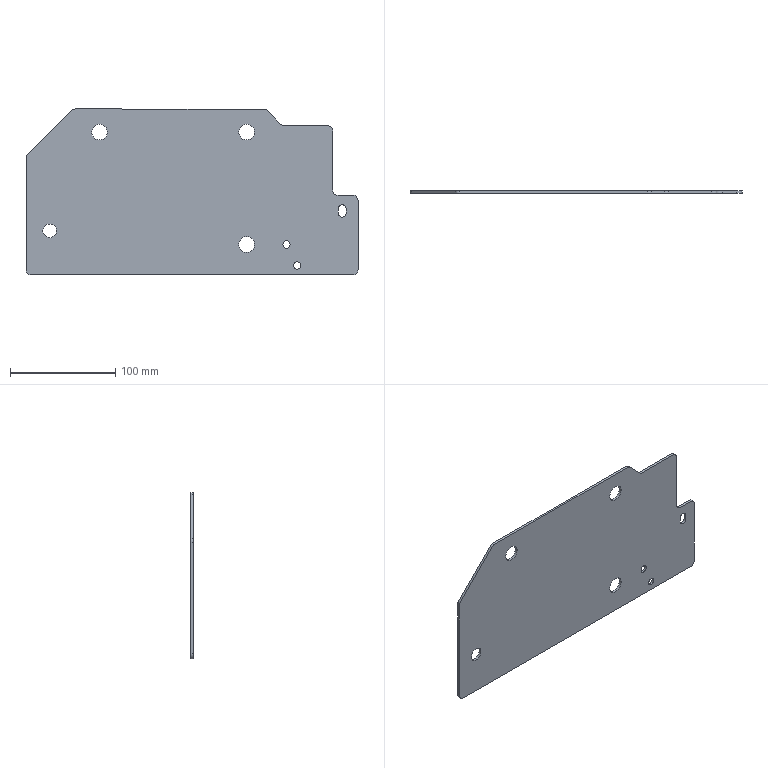Part | SolidWorks | features FlatPattern 1, SMBaseFlange 1, SheetMetal 1 | 1 solid | 37 faces | box 316 x 2.3 x 158 mm | volume 104007 mm3 | cylinder 24 | plane 13 | commonest cylinder face diameters 10 x9 15 x6 7 x4 7.3 x3 13 x2
STEP:
#1=CARTESIAN_POINT('',(258.,-2.3,5.5));
#2=VERTEX_POINT('',#1);
#3=CARTESIAN_POINT('',(258.,-2.3,12.5));
#4=VERTEX_POINT('',#3);
#5=CARTESIAN_POINT('',(258.,-2.3,9.));
#6=DIRECTION('',(0.,1.,0.));
#7=DIRECTION('',(0.,0.,1.));
#8=AXIS2_PLACEMENT_3D('',#5,#6,#7);
#9=CIRCLE('',#8,3.5);
#10=EDGE_CURVE('',#2,#4,#9,.T.);
#11=ORIENTED_EDGE('',*,*,#10,.F.);
#12=CARTESIAN_POINT('',(258.,0.,5.5));
#13=VERTEX_POINT('',#12);
#14=CARTESIAN_POINT('',(258.,-2.3,5.5));
#15=DIRECTION('',(0.,1.,0.));
#16=VECTOR('',#15,1000.);
#17=LINE('',#14,#16);
#18=EDGE_CURVE('',#2,#13,#17,.T.);
#19=ORIENTED_EDGE('',*,*,#18,.T.);
#20=CARTESIAN_POINT('',(258.,0.,12.5));
#21=VERTEX_POINT('',#20);
#22=CARTESIAN_POINT('',(258.,0.,9.));
#23=DIRECTION('',(0.,1.,0.));
#24=DIRECTION('',(0.,0.,1.));
#25=AXIS2_PLACEMENT_3D('',#22,#23,#24);
#26=CIRCLE('',#25,3.5);
#27=EDGE_CURVE('',#13,#21,#26,.T.);
#28=ORIENTED_EDGE('',*,*,#27,.T.);
#29=CARTESIAN_POINT('',(258.,-2.3,12.5));
#30=DIRECTION('',(0.,1.,0.));
#31=VECTOR('',#30,1000.);
#32=LINE('',#29,#31);
#33=EDGE_CURVE('',#4,#21,#32,.T.);
#34=ORIENTED_EDGE('',*,*,#33,.F.);
#35=EDGE_LOOP('',(#11,#19,#28,#34));
#36=FACE_OUTER_BOUND('',#35,.T.);
#37=CARTESIAN_POINT('',(258.,-2.3,9.));
#38=DIRECTION('',(0.,1.,0.));
#39=DIRECTION('',(0.,0.,1.));
#40=AXIS2_PLACEMENT_3D('',#37,#38,#39);
#41=CYLINDRICAL_SURFACE('',#40,3.5);
#42=ADVANCED_FACE('',(#36),#41,.F.);
#43=CARTESIAN_POINT('',(22.5,-2.3,35.5));
#44=VERTEX_POINT('',#43);
#45=CARTESIAN_POINT('',(22.5,-2.3,48.5));
#46=VERTEX_POINT('',#45);
#47=CARTESIAN_POINT('',(22.5,-2.3,42.));
#48=DIRECTION('',(0.,1.,0.));
#49=DIRECTION('',(0.,0.,1.));
#50=AXIS2_PLACEMENT_3D('',#47,#48,#49);
#51=CIRCLE('',#50,6.5);
#52=EDGE_CURVE('',#44,#46,#51,.T.);
#53=ORIENTED_EDGE('',*,*,#52,.F.);
#54=CARTESIAN_POINT('',(22.5,0.,35.5));
#55=VERTEX_POINT('',#54);
#56=CARTESIAN_POINT('',(22.5,-2.3,35.5));
#57=DIRECTION('',(0.,1.,0.));
#58=VECTOR('',#57,1000.);
#59=LINE('',#56,#58);
#60=EDGE_CURVE('',#44,#55,#59,.T.);
#61=ORIENTED_EDGE('',*,*,#60,.T.);
#62=CARTESIAN_POINT('',(22.5,0.,48.5));
#63=VERTEX_POINT('',#62);
#64=CARTESIAN_POINT('',(22.5,0.,42.));
#65=DIRECTION('',(0.,1.,0.));
#66=DIRECTION('',(0.,0.,1.));
#67=AXIS2_PLACEMENT_3D('',#64,#65,#66);
#68=CIRCLE('',#67,6.5);
#69=EDGE_CURVE('',#55,#63,#68,.T.);
#70=ORIENTED_EDGE('',*,*,#69,.T.);
#71=CARTESIAN_POINT('',(22.5,-2.3,48.5));
#72=DIRECTION('',(0.,1.,0.));
#73=VECTOR('',#72,1000.);
#74=LINE('',#71,#73);
#75=EDGE_CURVE('',#46,#63,#74,.T.);
#76=ORIENTED_EDGE('',*,*,#75,.F.);
#77=EDGE_LOOP('',(#53,#61,#70,#76));
#78=FACE_OUTER_BOUND('',#77,.T.);
#79=CARTESIAN_POINT('',(22.5,-2.3,42.));
#80=DIRECTION('',(0.,1.,0.));
#81=DIRECTION('',(0.,0.,1.));
#82=AXIS2_PLACEMENT_3D('',#79,#80,#81);
#83=CYLINDRICAL_SURFACE('',#82,6.5);
#84=ADVANCED_FACE('',(#78),#83,.F.);
#85=CARTESIAN_POINT('',(248.,-2.3,25.5));
#86=VERTEX_POINT('',#85);
#87=CARTESIAN_POINT('',(248.,-2.3,32.5));
#88=VERTEX_POINT('',#87);
#89=CARTESIAN_POINT('',(248.,-2.3,29.));
#90=DIRECTION('',(0.,1.,0.));
#91=DIRECTION('',(0.,0.,1.));
#92=AXIS2_PLACEMENT_3D('',#89,#90,#91);
#93=CIRCLE('',#92,3.5);
#94=EDGE_CURVE('',#86,#88,#93,.T.);
#95=ORIENTED_EDGE('',*,*,#94,.F.);
#96=CARTESIAN_POINT('',(248.,0.,25.5));
#97=VERTEX_POINT('',#96);
#98=CARTESIAN_POINT('',(248.,-2.3,25.5));
#99=DIRECTION('',(0.,1.,0.));
#100=VECTOR('',#99,1000.);
#101=LINE('',#98,#100);
#102=EDGE_CURVE('',#86,#97,#101,.T.);
#103=ORIENTED_EDGE('',*,*,#102,.T.);
#104=CARTESIAN_POINT('',(248.,0.,32.5));
#105=VERTEX_POINT('',#104);
#106=CARTESIAN_POINT('',(248.,0.,29.));
#107=DIRECTION('',(0.,1.,0.));
#108=DIRECTION('',(0.,0.,1.));
#109=AXIS2_PLACEMENT_3D('',#106,#107,#108);
#110=CIRCLE('',#109,3.5);
#111=EDGE_CURVE('',#97,#105,#110,.T.);
#112=ORIENTED_EDGE('',*,*,#111,.T.);
#113=CARTESIAN_POINT('',(248.,-2.3,32.5));
#114=DIRECTION('',(0.,1.,0.));
#115=VECTOR('',#114,1000.);
#116=LINE('',#113,#115);
#117=EDGE_CURVE('',#88,#105,#116,.T.);
#118=ORIENTED_EDGE('',*,*,#117,.F.);
#119=EDGE_LOOP('',(#95,#103,#112,#118));
#120=FACE_OUTER_BOUND('',#119,.T.);
#121=CARTESIAN_POINT('',(248.,-2.3,29.));
#122=DIRECTION('',(0.,1.,0.));
#123=DIRECTION('',(0.,0.,1.));
#124=AXIS2_PLACEMENT_3D('',#121,#122,#123);
#125=CYLINDRICAL_SURFACE('',#124,3.5);
#126=ADVANCED_FACE('',(#120),#125,.F.);
#127=CARTESIAN_POINT('',(70.,-2.3,128.5));
#128=VERTEX_POINT('',#127);
#129=CARTESIAN_POINT('',(70.,-2.3,143.5));
#130=VERTEX_POINT('',#129);
#131=CARTESIAN_POINT('',(70.,-2.3,136.));
#132=DIRECTION('',(0.,1.,0.));
#133=DIRECTION('',(0.,0.,1.));
#134=AXIS2_PLACEMENT_3D('',#131,#132,#133);
#135=CIRCLE('',#134,7.5);
#136=EDGE_CURVE('',#128,#130,#135,.T.);
#137=ORIENTED_EDGE('',*,*,#136,.F.);
#138=CARTESIAN_POINT('',(70.,0.,128.5));
#139=VERTEX_POINT('',#138);
#140=CARTESIAN_POINT('',(70.,-2.3,128.5));
#141=DIRECTION('',(0.,1.,0.));
#142=VECTOR('',#141,1000.);
#143=LINE('',#140,#142);
#144=EDGE_CURVE('',#128,#139,#143,.T.);
#145=ORIENTED_EDGE('',*,*,#144,.T.);
#146=CARTESIAN_POINT('',(70.,0.,143.5));
#147=VERTEX_POINT('',#146);
#148=CARTESIAN_POINT('',(70.,0.,136.));
#149=DIRECTION('',(0.,1.,0.));
#150=DIRECTION('',(0.,0.,1.));
#151=AXIS2_PLACEMENT_3D('',#148,#149,#150);
#152=CIRCLE('',#151,7.5);
#153=EDGE_CURVE('',#139,#147,#152,.T.);
#154=ORIENTED_EDGE('',*,*,#153,.T.);
#155=CARTESIAN_POINT('',(70.,-2.3,143.5));
#156=DIRECTION('',(0.,1.,0.));
#157=VECTOR('',#156,1000.);
#158=LINE('',#155,#157);
#159=EDGE_CURVE('',#130,#147,#158,.T.);
#160=ORIENTED_EDGE('',*,*,#159,.F.);
#161=EDGE_LOOP('',(#137,#145,#154,#160));
#162=FACE_OUTER_BOUND('',#161,.T.);
#163=CARTESIAN_POINT('',(70.,-2.3,136.));
#164=DIRECTION('',(0.,1.,0.));
#165=DIRECTION('',(0.,0.,1.));
#166=AXIS2_PLACEMENT_3D('',#163,#164,#165);
#167=CYLINDRICAL_SURFACE('',#166,7.5);
#168=ADVANCED_FACE('',(#162),#167,.F.);
#169=CARTESIAN_POINT('',(210.,-2.3,21.5));
#170=VERTEX_POINT('',#169);
#171=CARTESIAN_POINT('',(210.,-2.3,36.5));
#172=VERTEX_POINT('',#171);
#173=CARTESIAN_POINT('',(210.,-2.3,29.));
#174=DIRECTION('',(0.,1.,0.));
#175=DIRECTION('',(0.,0.,1.));
#176=AXIS2_PLACEMENT_3D('',#173,#174,#175);
#177=CIRCLE('',#176,7.5);
#178=EDGE_CURVE('',#170,#172,#177,.T.);
#179=ORIENTED_EDGE('',*,*,#178,.F.);
#180=CARTESIAN_POINT('',(210.,0.,21.5));
#181=VERTEX_POINT('',#180);
#182=CARTESIAN_POINT('',(210.,-2.3,21.5));
#183=DIRECTION('',(0.,1.,0.));
#184=VECTOR('',#183,1000.);
#185=LINE('',#182,#184);
#186=EDGE_CURVE('',#170,#181,#185,.T.);
#187=ORIENTED_EDGE('',*,*,#186,.T.);
#188=CARTESIAN_POINT('',(210.,0.,36.5));
#189=VERTEX_POINT('',#188);
#190=CARTESIAN_POINT('',(210.,0.,29.));
#191=DIRECTION('',(0.,1.,0.));
#192=DIRECTION('',(0.,0.,1.));
#193=AXIS2_PLACEMENT_3D('',#190,#191,#192);
#194=CIRCLE('',#193,7.5);
#195=EDGE_CURVE('',#181,#189,#194,.T.);
#196=ORIENTED_EDGE('',*,*,#195,.T.);
#197=CARTESIAN_POINT('',(210.,-2.3,36.5));
#198=DIRECTION('',(0.,1.,0.));
#199=VECTOR('',#198,1000.);
#200=LINE('',#197,#199);
#201=EDGE_CURVE('',#172,#189,#200,.T.);
#202=ORIENTED_EDGE('',*,*,#201,.F.);
#203=EDGE_LOOP('',(#179,#187,#196,#202));
#204=FACE_OUTER_BOUND('',#203,.T.);
#205=CARTESIAN_POINT('',(210.,-2.3,29.));
#206=DIRECTION('',(0.,1.,0.));
#207=DIRECTION('',(0.,0.,1.));
#208=AXIS2_PLACEMENT_3D('',#205,#206,#207);
#209=CYLINDRICAL_SURFACE('',#208,7.5);
#210=ADVANCED_FACE('',(#204),#209,.F.);
#211=CARTESIAN_POINT('',(210.,-2.3,128.5));
#212=VERTEX_POINT('',#211);
#213=CARTESIAN_POINT('',(210.,-2.3,143.5));
#214=VERTEX_POINT('',#213);
#215=CARTESIAN_POINT('',(210.,-2.3,136.));
#216=DIRECTION('',(0.,1.,0.));
#217=DIRECTION('',(0.,0.,1.));
#218=AXIS2_PLACEMENT_3D('',#215,#216,#217);
#219=CIRCLE('',#218,7.5);
#220=EDGE_CURVE('',#212,#214,#219,.T.);
#221=ORIENTED_EDGE('',*,*,#220,.F.);
#222=CARTESIAN_POINT('',(210.,0.,128.5));
#223=VERTEX_POINT('',#222);
#224=CARTESIAN_POINT('',(210.,-2.3,128.5));
#225=DIRECTION('',(0.,1.,0.));
#226=VECTOR('',#225,1000.);
#227=LINE('',#224,#226);
#228=EDGE_CURVE('',#212,#223,#227,.T.);
#229=ORIENTED_EDGE('',*,*,#228,.T.);
#230=CARTESIAN_POINT('',(210.,0.,143.5));
#231=VERTEX_POINT('',#230);
#232=CARTESIAN_POINT('',(210.,0.,136.));
#233=DIRECTION('',(0.,1.,0.));
#234=DIRECTION('',(0.,0.,1.));
#235=AXIS2_PLACEMENT_3D('',#232,#233,#234);
#236=CIRCLE('',#235,7.5);
#237=EDGE_CURVE('',#223,#231,#236,.T.);
#238=ORIENTED_EDGE('',*,*,#237,.T.);
#239=CARTESIAN_POINT('',(210.,-2.3,143.5));
#240=DIRECTION('',(0.,1.,0.));
#241=VECTOR('',#240,1000.);
#242=LINE('',#239,#241);
#243=EDGE_CURVE('',#214,#231,#242,.T.);
#244=ORIENTED_EDGE('',*,*,#243,.F.);
#245=EDGE_LOOP('',(#221,#229,#238,#244));
#246=FACE_OUTER_BOUND('',#245,.T.);
#247=CARTESIAN_POINT('',(210.,-2.3,136.));
#248=DIRECTION('',(0.,1.,0.));
#249=DIRECTION('',(0.,0.,1.));
#250=AXIS2_PLACEMENT_3D('',#247,#248,#249);
#251=CYLINDRICAL_SURFACE('',#250,7.5);
#252=ADVANCED_FACE('',(#246),#251,.F.);
#253=CARTESIAN_POINT('',(301.,-2.3,66.85));
#254=VERTEX_POINT('',#253);
#255=CARTESIAN_POINT('',(304.65,-2.3,63.2));
#256=VERTEX_POINT('',#255);
#257=CARTESIAN_POINT('',(301.,-2.3,63.2));
#258=DIRECTION('',(0.,1.,0.));
#259=DIRECTION('',(0.,0.,1.));
#260=AXIS2_PLACEMENT_3D('',#257,#258,#259);
#261=CIRCLE('',#260,3.65);
#262=EDGE_CURVE('',#254,#256,#261,.T.);
#263=ORIENTED_EDGE('',*,*,#262,.F.);
#264=CARTESIAN_POINT('',(301.,0.,66.85));
#265=VERTEX_POINT('',#264);
#266=CARTESIAN_POINT('',(301.,-2.3,66.85));
#267=DIRECTION('',(0.,1.,0.));
#268=VECTOR('',#267,1000.);
#269=LINE('',#266,#268);
#270=EDGE_CURVE('',#254,#265,#269,.T.);
#271=ORIENTED_EDGE('',*,*,#270,.T.);
#272=CARTESIAN_POINT('',(304.65,0.,63.2));
#273=VERTEX_POINT('',#272);
#274=CARTESIAN_POINT('',(301.,0.,63.2));
#275=DIRECTION('',(0.,1.,0.));
#276=DIRECTION('',(0.,0.,1.));
#277=AXIS2_PLACEMENT_3D('',#274,#275,#276);
#278=CIRCLE('',#277,3.65);
#279=EDGE_CURVE('',#265,#273,#278,.T.);
#280=ORIENTED_EDGE('',*,*,#279,.T.);
#281=CARTESIAN_POINT('',(304.65,-2.3,63.2));
#282=DIRECTION('',(0.,1.,0.));
#283=VECTOR('',#282,1000.);
#284=LINE('',#281,#283);
#285=EDGE_CURVE('',#256,#273,#284,.T.);
#286=ORIENTED_EDGE('',*,*,#285,.F.);
#287=EDGE_LOOP('',(#263,#271,#280,#286));
#288=FACE_OUTER_BOUND('',#287,.T.);
#289=CARTESIAN_POINT('',(301.,-2.3,63.2));
#290=DIRECTION('',(0.,1.,0.));
#291=DIRECTION('',(0.,0.,1.));
#292=AXIS2_PLACEMENT_3D('',#289,#290,#291);
#293=CYLINDRICAL_SURFACE('',#292,3.65);
#294=ADVANCED_FACE('',(#288),#293,.F.);
#295=CARTESIAN_POINT('',(316.,0.,5.));
#296=VERTEX_POINT('',#295);
#297=CARTESIAN_POINT('',(311.,0.,0.));
#298=VERTEX_POINT('',#297);
#299=CARTESIAN_POINT('',(311.,0.,5.));
#300=DIRECTION('',(0.,1.,0.));
#301=DIRECTION('',(0.,0.,-1.));
#302=AXIS2_PLACEMENT_3D('',#299,#300,#301);
#303=CIRCLE('',#302,5.);
#304=EDGE_CURVE('',#296,#298,#303,.T.);
#305=ORIENTED_EDGE('',*,*,#304,.F.);
#306=CARTESIAN_POINT('',(316.,-2.3,5.));
#307=VERTEX_POINT('',#306);
#308=CARTESIAN_POINT('',(316.,-2.3,5.));
#309=DIRECTION('',(0.,1.,0.));
#310=VECTOR('',#309,1000.);
#311=LINE('',#308,#310);
#312=EDGE_CURVE('',#307,#296,#311,.T.);
#313=ORIENTED_EDGE('',*,*,#312,.F.);
#314=CARTESIAN_POINT('',(311.,-2.3,0.));
#315=VERTEX_POINT('',#314);
#316=CARTESIAN_POINT('',(311.,-2.3,5.));
#317=DIRECTION('',(0.,1.,0.));
#318=DIRECTION('',(0.,0.,-1.));
#319=AXIS2_PLACEMENT_3D('',#316,#317,#318);
#320=CIRCLE('',#319,5.);
#321=EDGE_CURVE('',#307,#315,#320,.T.);
#322=ORIENTED_EDGE('',*,*,#321,.T.);
#323=CARTESIAN_POINT('',(311.,-2.3,0.));
#324=DIRECTION('',(0.,1.,0.));
#325=VECTOR('',#324,1000.);
#326=LINE('',#323,#325);
#327=EDGE_CURVE('',#315,#298,#326,.T.);
#328=ORIENTED_EDGE('',*,*,#327,.T.);
#329=EDGE_LOOP('',(#305,#313,#322,#328));
#330=FACE_OUTER_BOUND('',#329,.T.);
#331=CARTESIAN_POINT('',(311.,-2.3,5.));
#332=DIRECTION('',(0.,1.,0.));
#333=DIRECTION('',(0.,0.,1.));
#334=AXIS2_PLACEMENT_3D('',#331,#332,#333);
#335=CYLINDRICAL_SURFACE('',#334,5.);
#336=ADVANCED_FACE('',(#330),#335,.T.);
#337=CARTESIAN_POINT('',(316.,0.,71.));
#338=VERTEX_POINT('',#337);
#339=CARTESIAN_POINT('',(316.,0.,5.));
#340=DIRECTION('',(0.,0.,-1.));
#341=VECTOR('',#340,1000.);
#342=LINE('',#339,#341);
#343=EDGE_CURVE('',#338,#296,#342,.T.);
#344=ORIENTED_EDGE('',*,*,#343,.F.);
#345=CARTESIAN_POINT('',(316.,-2.3,71.));
#346=VERTEX_POINT('',#345);
#347=CARTESIAN_POINT('',(316.,-2.3,71.));
#348=DIRECTION('',(0.,1.,0.));
#349=VECTOR('',#348,1000.);
#350=LINE('',#347,#349);
#351=EDGE_CURVE('',#346,#338,#350,.T.);
#352=ORIENTED_EDGE('',*,*,#351,.F.);
#353=CARTESIAN_POINT('',(316.,-2.3,5.));
#354=DIRECTION('',(0.,0.,-1.));
#355=VECTOR('',#354,1000.);
#356=LINE('',#353,#355);
#357=EDGE_CURVE('',#346,#307,#356,.T.);
#358=ORIENTED_EDGE('',*,*,#357,.T.);
#359=ORIENTED_EDGE('',*,*,#312,.T.);
#360=EDGE_LOOP('',(#344,#352,#358,#359));
#361=FACE_OUTER_BOUND('',#360,.T.);
#362=CARTESIAN_POINT('',(316.,-2.3,5.));
#363=DIRECTION('',(1.,0.,0.));
#364=DIRECTION('',(0.,0.,-1.));
#365=AXIS2_PLACEMENT_3D('',#362,#363,#364);
#366=PLANE('',#365);
#367=ADVANCED_FACE('',(#361),#366,.T.);
#368=CARTESIAN_POINT('',(311.,0.,76.));
#369=VERTEX_POINT('',#368);
#370=CARTESIAN_POINT('',(311.,0.,71.));
#371=DIRECTION('',(0.,1.,0.));
#372=DIRECTION('',(0.,0.,1.));
#373=AXIS2_PLACEMENT_3D('',#370,#371,#372);
#374=CIRCLE('',#373,5.);
#375=EDGE_CURVE('',#369,#338,#374,.T.);
#376=ORIENTED_EDGE('',*,*,#375,.F.);
#377=CARTESIAN_POINT('',(311.,-2.3,76.));
#378=VERTEX_POINT('',#377);
#379=CARTESIAN_POINT('',(311.,-2.3,76.));
#380=DIRECTION('',(0.,1.,0.));
#381=VECTOR('',#380,1000.);
#382=LINE('',#379,#381);
#383=EDGE_CURVE('',#378,#369,#382,.T.);
#384=ORIENTED_EDGE('',*,*,#383,.F.);
#385=CARTESIAN_POINT('',(311.,-2.3,71.));
#386=DIRECTION('',(0.,1.,0.));
#387=DIRECTION('',(0.,0.,1.));
#388=AXIS2_PLACEMENT_3D('',#385,#386,#387);
#389=CIRCLE('',#388,5.);
#390=EDGE_CURVE('',#378,#346,#389,.T.);
#391=ORIENTED_EDGE('',*,*,#390,.T.);
#392=ORIENTED_EDGE('',*,*,#351,.T.);
#393=EDGE_LOOP('',(#376,#384,#391,#392));
#394=FACE_OUTER_BOUND('',#393,.T.);
#395=CARTESIAN_POINT('',(311.,-2.3,71.));
#396=DIRECTION('',(0.,1.,0.));
#397=DIRECTION('',(0.,0.,1.));
#398=AXIS2_PLACEMENT_3D('',#395,#396,#397);
#399=CYLINDRICAL_SURFACE('',#398,5.);
#400=ADVANCED_FACE('',(#394),#399,.T.);
#401=CARTESIAN_POINT('',(297.,0.,76.));
#402=VERTEX_POINT('',#401);
#403=CARTESIAN_POINT('',(311.,0.,76.));
#404=DIRECTION('',(1.,0.,0.));
#405=VECTOR('',#404,1000.);
#406=LINE('',#403,#405);
#407=EDGE_CURVE('',#402,#369,#406,.T.);
#408=ORIENTED_EDGE('',*,*,#407,.F.);
#409=CARTESIAN_POINT('',(297.,-2.3,76.));
#410=VERTEX_POINT('',#409);
#411=CARTESIAN_POINT('',(297.,-2.3,76.));
#412=DIRECTION('',(0.,1.,0.));
#413=VECTOR('',#412,1000.);
#414=LINE('',#411,#413);
#415=EDGE_CURVE('',#410,#402,#414,.T.);
#416=ORIENTED_EDGE('',*,*,#415,.F.);
#417=CARTESIAN_POINT('',(311.,-2.3,76.));
#418=DIRECTION('',(1.,0.,0.));
#419=VECTOR('',#418,1000.);
#420=LINE('',#417,#419);
#421=EDGE_CURVE('',#410,#378,#420,.T.);
#422=ORIENTED_EDGE('',*,*,#421,.T.);
#423=ORIENTED_EDGE('',*,*,#383,.T.);
#424=EDGE_LOOP('',(#408,#416,#422,#423));
#425=FACE_OUTER_BOUND('',#424,.T.);
#426=CARTESIAN_POINT('',(311.,-2.3,76.));
#427=DIRECTION('',(0.,0.,1.));
#428=DIRECTION('',(1.,0.,0.));
#429=AXIS2_PLACEMENT_3D('',#426,#427,#428);
#430=PLANE('',#429);
#431=ADVANCED_FACE('',(#425),#430,.T.);
#432=CARTESIAN_POINT('',(292.,0.,81.));
#433=VERTEX_POINT('',#432);
#434=CARTESIAN_POINT('',(297.,0.,81.));
#435=DIRECTION('',(0.,-1.,0.));
#436=DIRECTION('',(0.,0.,1.));
#437=AXIS2_PLACEMENT_3D('',#434,#435,#436);
#438=CIRCLE('',#437,5.);
#439=EDGE_CURVE('',#433,#402,#438,.T.);
#440=ORIENTED_EDGE('',*,*,#439,.F.);
#441=CARTESIAN_POINT('',(292.,-2.3,81.));
#442=VERTEX_POINT('',#441);
#443=CARTESIAN_POINT('',(292.,-2.3,81.));
#444=DIRECTION('',(0.,1.,0.));
#445=VECTOR('',#444,1000.);
#446=LINE('',#443,#445);
#447=EDGE_CURVE('',#442,#433,#446,.T.);
#448=ORIENTED_EDGE('',*,*,#447,.F.);
#449=CARTESIAN_POINT('',(297.,-2.3,81.));
#450=DIRECTION('',(0.,-1.,0.));
#451=DIRECTION('',(0.,0.,1.));
#452=AXIS2_PLACEMENT_3D('',#449,#450,#451);
#453=CIRCLE('',#452,5.);
#454=EDGE_CURVE('',#442,#410,#453,.T.);
#455=ORIENTED_EDGE('',*,*,#454,.T.);
#456=ORIENTED_EDGE('',*,*,#415,.T.);
#457=EDGE_LOOP('',(#440,#448,#455,#456));
#458=FACE_OUTER_BOUND('',#457,.T.);
#459=CARTESIAN_POINT('',(297.,-2.3,81.));
#460=DIRECTION('',(0.,1.,0.));
#461=DIRECTION('',(0.,0.,1.));
#462=AXIS2_PLACEMENT_3D('',#459,#460,#461);
#463=CYLINDRICAL_SURFACE('',#462,5.);
#464=ADVANCED_FACE('',(#458),#463,.F.);
#465=CARTESIAN_POINT('',(292.,0.,137.));
#466=VERTEX_POINT('',#465);
#467=CARTESIAN_POINT('',(292.,0.,81.));
#468=DIRECTION('',(0.,0.,-1.));
#469=VECTOR('',#468,1000.);
#470=LINE('',#467,#469);
#471=EDGE_CURVE('',#466,#433,#470,.T.);
#472=ORIENTED_EDGE('',*,*,#471,.F.);
#473=CARTESIAN_POINT('',(292.,-2.3,137.));
#474=VERTEX_POINT('',#473);
#475=CARTESIAN_POINT('',(292.,-2.3,137.));
#476=DIRECTION('',(0.,1.,0.));
#477=VECTOR('',#476,1000.);
#478=LINE('',#475,#477);
#479=EDGE_CURVE('',#474,#466,#478,.T.);
#480=ORIENTED_EDGE('',*,*,#479,.F.);
#481=CARTESIAN_POINT('',(292.,-2.3,81.));
#482=DIRECTION('',(0.,0.,-1.));
#483=VECTOR('',#482,1000.);
#484=LINE('',#481,#483);
#485=EDGE_CURVE('',#474,#442,#484,.T.);
#486=ORIENTED_EDGE('',*,*,#485,.T.);
#487=ORIENTED_EDGE('',*,*,#447,.T.);
#488=EDGE_LOOP('',(#472,#480,#486,#487));
#489=FACE_OUTER_BOUND('',#488,.T.);
#490=CARTESIAN_POINT('',(292.,-2.3,81.));
#491=DIRECTION('',(1.,0.,0.));
#492=DIRECTION('',(0.,0.,-1.));
#493=AXIS2_PLACEMENT_3D('',#490,#491,#492);
#494=PLANE('',#493);
#495=ADVANCED_FACE('',(#489),#494,.T.);
#496=CARTESIAN_POINT('',(287.,0.,142.));
#497=VERTEX_POINT('',#496);
#498=CARTESIAN_POINT('',(287.,0.,137.));
#499=DIRECTION('',(0.,1.,0.));
#500=DIRECTION('',(0.,0.,-1.));
#501=AXIS2_PLACEMENT_3D('',#498,#499,#500);
#502=CIRCLE('',#501,5.);
#503=EDGE_CURVE('',#497,#466,#502,.T.);
#504=ORIENTED_EDGE('',*,*,#503,.F.);
#505=CARTESIAN_POINT('',(287.,-2.3,142.));
#506=VERTEX_POINT('',#505);
#507=CARTESIAN_POINT('',(287.,-2.3,142.));
#508=DIRECTION('',(0.,1.,0.));
#509=VECTOR('',#508,1000.);
#510=LINE('',#507,#509);
#511=EDGE_CURVE('',#506,#497,#510,.T.);
#512=ORIENTED_EDGE('',*,*,#511,.F.);
#513=CARTESIAN_POINT('',(287.,-2.3,137.));
#514=DIRECTION('',(0.,1.,0.));
#515=DIRECTION('',(0.,0.,-1.));
#516=AXIS2_PLACEMENT_3D('',#513,#514,#515);
#517=CIRCLE('',#516,5.);
#518=EDGE_CURVE('',#506,#474,#517,.T.);
#519=ORIENTED_EDGE('',*,*,#518,.T.);
#520=ORIENTED_EDGE('',*,*,#479,.T.);
#521=EDGE_LOOP('',(#504,#512,#519,#520));
#522=FACE_OUTER_BOUND('',#521,.T.);
#523=CARTESIAN_POINT('',(287.,-2.3,137.));
#524=DIRECTION('',(0.,1.,0.));
#525=DIRECTION('',(0.,0.,1.));
#526=AXIS2_PLACEMENT_3D('',#523,#524,#525);
#527=CYLINDRICAL_SURFACE('',#526,5.);
#528=ADVANCED_FACE('',(#522),#527,.T.);
#529=CARTESIAN_POINT('',(246.071,0.,142.));
#530=VERTEX_POINT('',#529);
#531=CARTESIAN_POINT('',(287.,0.,142.));
#532=DIRECTION('',(1.,0.,0.));
#533=VECTOR('',#532,1000.);
#534=LINE('',#531,#533);
#535=EDGE_CURVE('',#530,#497,#534,.T.);
#536=ORIENTED_EDGE('',*,*,#535,.F.);
#537=CARTESIAN_POINT('',(246.071,-2.3,142.));
#538=VERTEX_POINT('',#537);
#539=CARTESIAN_POINT('',(246.071,-2.3,142.));
#540=DIRECTION('',(0.,1.,0.));
#541=VECTOR('',#540,1000.);
#542=LINE('',#539,#541);
#543=EDGE_CURVE('',#538,#530,#542,.T.);
#544=ORIENTED_EDGE('',*,*,#543,.F.);
#545=CARTESIAN_POINT('',(287.,-2.3,142.));
#546=DIRECTION('',(1.,0.,0.));
#547=VECTOR('',#546,1000.);
#548=LINE('',#545,#547);
#549=EDGE_CURVE('',#538,#506,#548,.T.);
#550=ORIENTED_EDGE('',*,*,#549,.T.);
#551=ORIENTED_EDGE('',*,*,#511,.T.);
#552=EDGE_LOOP('',(#536,#544,#550,#551));
#553=FACE_OUTER_BOUND('',#552,.T.);
#554=CARTESIAN_POINT('',(287.,-2.3,142.));
#555=DIRECTION('',(0.,0.,1.));
#556=DIRECTION('',(1.,0.,0.));
#557=AXIS2_PLACEMENT_3D('',#554,#555,#556);
#558=PLANE('',#557);
#559=ADVANCED_FACE('',(#553),#558,.T.);
#560=CARTESIAN_POINT('',(242.536,0.,143.464));
#561=VERTEX_POINT('',#560);
#562=CARTESIAN_POINT('',(246.071,0.,147.));
#563=DIRECTION('',(0.,-1.,0.));
#564=DIRECTION('',(0.,0.,1.));
#565=AXIS2_PLACEMENT_3D('',#562,#563,#564);
#566=CIRCLE('',#565,5.);
#567=EDGE_CURVE('',#561,#530,#566,.T.);
#568=ORIENTED_EDGE('',*,*,#567,.F.);
#569=CARTESIAN_POINT('',(242.536,-2.3,143.464));
#570=VERTEX_POINT('',#569);
#571=CARTESIAN_POINT('',(242.536,-2.3,143.464));
#572=DIRECTION('',(0.,1.,0.));
#573=VECTOR('',#572,1000.);
#574=LINE('',#571,#573);
#575=EDGE_CURVE('',#570,#561,#574,.T.);
#576=ORIENTED_EDGE('',*,*,#575,.F.);
#577=CARTESIAN_POINT('',(246.071,-2.3,147.));
#578=DIRECTION('',(0.,-1.,0.));
#579=DIRECTION('',(0.,0.,1.));
#580=AXIS2_PLACEMENT_3D('',#577,#578,#579);
#581=CIRCLE('',#580,5.);
#582=EDGE_CURVE('',#570,#538,#581,.T.);
#583=ORIENTED_EDGE('',*,*,#582,.T.);
#584=ORIENTED_EDGE('',*,*,#543,.T.);
#585=EDGE_LOOP('',(#568,#576,#583,#584));
#586=FACE_OUTER_BOUND('',#585,.T.);
#587=CARTESIAN_POINT('',(246.071,-2.3,147.));
#588=DIRECTION('',(0.,1.,0.));
#589=DIRECTION('',(0.,0.,1.));
#590=AXIS2_PLACEMENT_3D('',#587,#588,#589);
#591=CYLINDRICAL_SURFACE('',#590,5.);
#592=ADVANCED_FACE('',(#586),#591,.F.);
#593=CARTESIAN_POINT('',(229.464,0.,156.536));
#594=VERTEX_POINT('',#593);
#595=CARTESIAN_POINT('',(242.536,0.,143.464));
#596=DIRECTION('',(0.7071,0.,-0.7071));
#597=VECTOR('',#596,1000.);
#598=LINE('',#595,#597);
#599=EDGE_CURVE('',#594,#561,#598,.T.);
#600=ORIENTED_EDGE('',*,*,#599,.F.);
#601=CARTESIAN_POINT('',(229.464,-2.3,156.536));
#602=VERTEX_POINT('',#601);
#603=CARTESIAN_POINT('',(229.464,-2.3,156.536));
#604=DIRECTION('',(0.,1.,0.));
#605=VECTOR('',#604,1000.);
#606=LINE('',#603,#605);
#607=EDGE_CURVE('',#602,#594,#606,.T.);
#608=ORIENTED_EDGE('',*,*,#607,.F.);
#609=CARTESIAN_POINT('',(242.536,-2.3,143.464));
#610=DIRECTION('',(0.7071,0.,-0.7071));
#611=VECTOR('',#610,1000.);
#612=LINE('',#609,#611);
#613=EDGE_CURVE('',#602,#570,#612,.T.);
#614=ORIENTED_EDGE('',*,*,#613,.T.);
#615=ORIENTED_EDGE('',*,*,#575,.T.);
#616=EDGE_LOOP('',(#600,#608,#614,#615));
#617=FACE_OUTER_BOUND('',#616,.T.);
#618=CARTESIAN_POINT('',(242.536,-2.3,143.464));
#619=DIRECTION('',(0.7071,0.,0.7071));
#620=DIRECTION('',(0.7071,0.,-0.7071));
#621=AXIS2_PLACEMENT_3D('',#618,#619,#620);
#622=PLANE('',#621);
#623=ADVANCED_FACE('',(#617),#622,.T.);
#624=CARTESIAN_POINT('',(225.929,0.,158.));
#625=VERTEX_POINT('',#624);
#626=CARTESIAN_POINT('',(225.929,0.,153.));
#627=DIRECTION('',(0.,1.,0.));
#628=DIRECTION('',(0.,0.,-1.));
#629=AXIS2_PLACEMENT_3D('',#626,#627,#628);
#630=CIRCLE('',#629,5.);
#631=EDGE_CURVE('',#625,#594,#630,.T.);
#632=ORIENTED_EDGE('',*,*,#631,.F.);
#633=CARTESIAN_POINT('',(225.929,-2.3,158.));
#634=VERTEX_POINT('',#633);
#635=CARTESIAN_POINT('',(225.929,-2.3,158.));
#636=DIRECTION('',(0.,1.,0.));
#637=VECTOR('',#636,1000.);
#638=LINE('',#635,#637);
#639=EDGE_CURVE('',#634,#625,#638,.T.);
#640=ORIENTED_EDGE('',*,*,#639,.F.);
#641=CARTESIAN_POINT('',(225.929,-2.3,153.));
#642=DIRECTION('',(0.,1.,0.));
#643=DIRECTION('',(0.,0.,-1.));
#644=AXIS2_PLACEMENT_3D('',#641,#642,#643);
#645=CIRCLE('',#644,5.);
#646=EDGE_CURVE('',#634,#602,#645,.T.);
#647=ORIENTED_EDGE('',*,*,#646,.T.);
#648=ORIENTED_EDGE('',*,*,#607,.T.);
#649=EDGE_LOOP('',(#632,#640,#647,#648));
#650=FACE_OUTER_BOUND('',#649,.T.);
#651=CARTESIAN_POINT('',(225.929,-2.3,153.));
#652=DIRECTION('',(0.,1.,0.));
#653=DIRECTION('',(0.,0.,1.));
#654=AXIS2_PLACEMENT_3D('',#651,#652,#653);
#655=CYLINDRICAL_SURFACE('',#654,5.);
#656=ADVANCED_FACE('',(#650),#655,.T.);
#657=CARTESIAN_POINT('',(47.071,0.,158.));
#658=VERTEX_POINT('',#657);
#659=CARTESIAN_POINT('',(225.929,0.,158.));
#660=DIRECTION('',(1.,0.,0.));
#661=VECTOR('',#660,1000.);
#662=LINE('',#659,#661);
#663=EDGE_CURVE('',#658,#625,#662,.T.);
#664=ORIENTED_EDGE('',*,*,#663,.F.);
#665=CARTESIAN_POINT('',(47.071,-2.3,158.));
#666=VERTEX_POINT('',#665);
#667=CARTESIAN_POINT('',(47.071,-2.3,158.));
#668=DIRECTION('',(0.,1.,0.));
#669=VECTOR('',#668,1000.);
#670=LINE('',#667,#669);
#671=EDGE_CURVE('',#666,#658,#670,.T.);
#672=ORIENTED_EDGE('',*,*,#671,.F.);
#673=CARTESIAN_POINT('',(225.929,-2.3,158.));
#674=DIRECTION('',(1.,0.,0.));
#675=VECTOR('',#674,1000.);
#676=LINE('',#673,#675);
#677=EDGE_CURVE('',#666,#634,#676,.T.);
#678=ORIENTED_EDGE('',*,*,#677,.T.);
#679=ORIENTED_EDGE('',*,*,#639,.T.);
#680=EDGE_LOOP('',(#664,#672,#678,#679));
#681=FACE_OUTER_BOUND('',#680,.T.);
#682=CARTESIAN_POINT('',(225.929,-2.3,158.));
#683=DIRECTION('',(0.,0.,1.));
#684=DIRECTION('',(1.,0.,0.));
#685=AXIS2_PLACEMENT_3D('',#682,#683,#684);
#686=PLANE('',#685);
#687=ADVANCED_FACE('',(#681),#686,.T.);
#688=CARTESIAN_POINT('',(43.536,0.,156.536));
#689=VERTEX_POINT('',#688);
#690=CARTESIAN_POINT('',(47.071,0.,153.));
#691=DIRECTION('',(0.,1.,0.));
#692=DIRECTION('',(0.,0.,1.));
#693=AXIS2_PLACEMENT_3D('',#690,#691,#692);
#694=CIRCLE('',#693,5.);
#695=EDGE_CURVE('',#689,#658,#694,.T.);
#696=ORIENTED_EDGE('',*,*,#695,.F.);
#697=CARTESIAN_POINT('',(43.536,-2.3,156.536));
#698=VERTEX_POINT('',#697);
#699=CARTESIAN_POINT('',(43.536,-2.3,156.536));
#700=DIRECTION('',(0.,1.,0.));
#701=VECTOR('',#700,1000.);
#702=LINE('',#699,#701);
#703=EDGE_CURVE('',#698,#689,#702,.T.);
#704=ORIENTED_EDGE('',*,*,#703,.F.);
#705=CARTESIAN_POINT('',(47.071,-2.3,153.));
#706=DIRECTION('',(0.,1.,0.));
#707=DIRECTION('',(0.,0.,1.));
#708=AXIS2_PLACEMENT_3D('',#705,#706,#707);
#709=CIRCLE('',#708,5.);
#710=EDGE_CURVE('',#698,#666,#709,.T.);
#711=ORIENTED_EDGE('',*,*,#710,.T.);
#712=ORIENTED_EDGE('',*,*,#671,.T.);
#713=EDGE_LOOP('',(#696,#704,#711,#712));
#714=FACE_OUTER_BOUND('',#713,.T.);
#715=CARTESIAN_POINT('',(47.071,-2.3,153.));
#716=DIRECTION('',(0.,1.,0.));
#717=DIRECTION('',(0.,0.,1.));
#718=AXIS2_PLACEMENT_3D('',#715,#716,#717);
#719=CYLINDRICAL_SURFACE('',#718,5.);
#720=ADVANCED_FACE('',(#714),#719,.T.);
#721=CARTESIAN_POINT('',(1.464,0.,114.464));
#722=VERTEX_POINT('',#721);
#723=CARTESIAN_POINT('',(43.536,0.,156.536));
#724=DIRECTION('',(0.7071,0.,0.7071));
#725=VECTOR('',#724,1000.);
#726=LINE('',#723,#725);
#727=EDGE_CURVE('',#722,#689,#726,.T.);
#728=ORIENTED_EDGE('',*,*,#727,.F.);
#729=CARTESIAN_POINT('',(1.464,-2.3,114.464));
#730=VERTEX_POINT('',#729);
#731=CARTESIAN_POINT('',(1.464,-2.3,114.464));
#732=DIRECTION('',(0.,1.,0.));
#733=VECTOR('',#732,1000.);
#734=LINE('',#731,#733);
#735=EDGE_CURVE('',#730,#722,#734,.T.);
#736=ORIENTED_EDGE('',*,*,#735,.F.);
#737=CARTESIAN_POINT('',(43.536,-2.3,156.536));
#738=DIRECTION('',(0.7071,0.,0.7071));
#739=VECTOR('',#738,1000.);
#740=LINE('',#737,#739);
#741=EDGE_CURVE('',#730,#698,#740,.T.);
#742=ORIENTED_EDGE('',*,*,#741,.T.);
#743=ORIENTED_EDGE('',*,*,#703,.T.);
#744=EDGE_LOOP('',(#728,#736,#742,#743));
#745=FACE_OUTER_BOUND('',#744,.T.);
#746=CARTESIAN_POINT('',(43.536,-2.3,156.536));
#747=DIRECTION('',(-0.7071,0.,0.7071));
#748=DIRECTION('',(0.7071,0.,0.7071));
#749=AXIS2_PLACEMENT_3D('',#746,#747,#748);
#750=PLANE('',#749);
#751=ADVANCED_FACE('',(#745),#750,.T.);
#752=CARTESIAN_POINT('',(0.,0.,110.929));
#753=VERTEX_POINT('',#752);
#754=CARTESIAN_POINT('',(5.,0.,110.929));
#755=DIRECTION('',(0.,1.,0.));
#756=DIRECTION('',(0.,0.,-1.));
#757=AXIS2_PLACEMENT_3D('',#754,#755,#756);
#758=CIRCLE('',#757,5.);
#759=EDGE_CURVE('',#753,#722,#758,.T.);
#760=ORIENTED_EDGE('',*,*,#759,.F.);
#761=CARTESIAN_POINT('',(0.,-2.3,110.929));
#762=VERTEX_POINT('',#761);
#763=CARTESIAN_POINT('',(0.,-2.3,110.929));
#764=DIRECTION('',(0.,1.,0.));
#765=VECTOR('',#764,1000.);
#766=LINE('',#763,#765);
#767=EDGE_CURVE('',#762,#753,#766,.T.);
#768=ORIENTED_EDGE('',*,*,#767,.F.);
#769=CARTESIAN_POINT('',(5.,-2.3,110.929));
#770=DIRECTION('',(0.,1.,0.));
#771=DIRECTION('',(0.,0.,-1.));
#772=AXIS2_PLACEMENT_3D('',#769,#770,#771);
#773=CIRCLE('',#772,5.);
#774=EDGE_CURVE('',#762,#730,#773,.T.);
#775=ORIENTED_EDGE('',*,*,#774,.T.);
#776=ORIENTED_EDGE('',*,*,#735,.T.);
#777=EDGE_LOOP('',(#760,#768,#775,#776));
#778=FACE_OUTER_BOUND('',#777,.T.);
#779=CARTESIAN_POINT('',(5.,-2.3,110.929));
#780=DIRECTION('',(0.,1.,0.));
#781=DIRECTION('',(0.,0.,1.));
#782=AXIS2_PLACEMENT_3D('',#779,#780,#781);
#783=CYLINDRICAL_SURFACE('',#782,5.);
#784=ADVANCED_FACE('',(#778),#783,.T.);
#785=CARTESIAN_POINT('',(0.,0.,5.));
#786=VERTEX_POINT('',#785);
#787=CARTESIAN_POINT('',(0.,0.,110.929));
#788=DIRECTION('',(0.,0.,1.));
#789=VECTOR('',#788,1000.);
#790=LINE('',#787,#789);
#791=EDGE_CURVE('',#786,#753,#790,.T.);
#792=ORIENTED_EDGE('',*,*,#791,.F.);
#793=CARTESIAN_POINT('',(0.,-2.3,5.));
#794=VERTEX_POINT('',#793);
#795=CARTESIAN_POINT('',(0.,-2.3,5.));
#796=DIRECTION('',(0.,1.,0.));
#797=VECTOR('',#796,1000.);
#798=LINE('',#795,#797);
#799=EDGE_CURVE('',#794,#786,#798,.T.);
#800=ORIENTED_EDGE('',*,*,#799,.F.);
#801=CARTESIAN_POINT('',(0.,-2.3,110.929));
#802=DIRECTION('',(0.,0.,1.));
#803=VECTOR('',#802,1000.);
#804=LINE('',#801,#803);
#805=EDGE_CURVE('',#794,#762,#804,.T.);
#806=ORIENTED_EDGE('',*,*,#805,.T.);
#807=ORIENTED_EDGE('',*,*,#767,.T.);
#808=EDGE_LOOP('',(#792,#800,#806,#807));
#809=FACE_OUTER_BOUND('',#808,.T.);
#810=CARTESIAN_POINT('',(0.,-2.3,110.929));
#811=DIRECTION('',(-1.,0.,0.));
#812=DIRECTION('',(0.,0.,1.));
#813=AXIS2_PLACEMENT_3D('',#810,#811,#812);
#814=PLANE('',#813);
#815=ADVANCED_FACE('',(#809),#814,.T.);
#816=CARTESIAN_POINT('',(5.,0.,0.));
#817=VERTEX_POINT('',#816);
#818=CARTESIAN_POINT('',(5.,0.,5.));
#819=DIRECTION('',(0.,1.,0.));
#820=DIRECTION('',(0.,0.,1.));
#821=AXIS2_PLACEMENT_3D('',#818,#819,#820);
#822=CIRCLE('',#821,5.);
#823=EDGE_CURVE('',#817,#786,#822,.T.);
#824=ORIENTED_EDGE('',*,*,#823,.F.);
#825=CARTESIAN_POINT('',(5.,-2.3,0.));
#826=VERTEX_POINT('',#825);
#827=CARTESIAN_POINT('',(5.,-2.3,0.));
#828=DIRECTION('',(0.,1.,0.));
#829=VECTOR('',#828,1000.);
#830=LINE('',#827,#829);
#831=EDGE_CURVE('',#826,#817,#830,.T.);
#832=ORIENTED_EDGE('',*,*,#831,.F.);
#833=CARTESIAN_POINT('',(5.,-2.3,5.));
#834=DIRECTION('',(0.,1.,0.));
#835=DIRECTION('',(0.,0.,1.));
#836=AXIS2_PLACEMENT_3D('',#833,#834,#835);
#837=CIRCLE('',#836,5.);
#838=EDGE_CURVE('',#826,#794,#837,.T.);
#839=ORIENTED_EDGE('',*,*,#838,.T.);
#840=ORIENTED_EDGE('',*,*,#799,.T.);
#841=EDGE_LOOP('',(#824,#832,#839,#840));
#842=FACE_OUTER_BOUND('',#841,.T.);
#843=CARTESIAN_POINT('',(5.,-2.3,5.));
#844=DIRECTION('',(0.,1.,0.));
#845=DIRECTION('',(0.,0.,1.));
#846=AXIS2_PLACEMENT_3D('',#843,#844,#845);
#847=CYLINDRICAL_SURFACE('',#846,5.);
#848=ADVANCED_FACE('',(#842),#847,.T.);
#849=CARTESIAN_POINT('',(5.,0.,0.));
#850=DIRECTION('',(-1.,0.,0.));
#851=VECTOR('',#850,1000.);
#852=LINE('',#849,#851);
#853=EDGE_CURVE('',#298,#817,#852,.T.);
#854=ORIENTED_EDGE('',*,*,#853,.F.);
#855=ORIENTED_EDGE('',*,*,#327,.F.);
#856=CARTESIAN_POINT('',(5.,-2.3,0.));
#857=DIRECTION('',(-1.,0.,0.));
#858=VECTOR('',#857,1000.);
#859=LINE('',#856,#858);
#860=EDGE_CURVE('',#315,#826,#859,.T.);
#861=ORIENTED_EDGE('',*,*,#860,.T.);
#862=ORIENTED_EDGE('',*,*,#831,.T.);
#863=EDGE_LOOP('',(#854,#855,#861,#862));
#864=FACE_OUTER_BOUND('',#863,.T.);
#865=CARTESIAN_POINT('',(5.,-2.3,0.));
#866=DIRECTION('',(0.,0.,-1.));
#867=DIRECTION('',(-1.,0.,0.));
#868=AXIS2_PLACEMENT_3D('',#865,#866,#867);
#869=PLANE('',#868);
#870=ADVANCED_FACE('',(#864),#869,.T.);
#871=CARTESIAN_POINT('',(258.,-2.3,9.));
#872=DIRECTION('',(0.,1.,0.));
#873=DIRECTION('',(0.,0.,1.));
#874=AXIS2_PLACEMENT_3D('',#871,#872,#873);
#875=CIRCLE('',#874,3.5);
#876=EDGE_CURVE('',#4,#2,#875,.T.);
#877=ORIENTED_EDGE('',*,*,#876,.T.);
#878=ORIENTED_EDGE('',*,*,#10,.T.);
#879=EDGE_LOOP('',(#877,#878));
#880=FACE_BOUND('',#879,.T.);
#881=CARTESIAN_POINT('',(22.5,-2.3,42.));
#882=DIRECTION('',(0.,1.,0.));
#883=DIRECTION('',(0.,0.,1.));
#884=AXIS2_PLACEMENT_3D('',#881,#882,#883);
#885=CIRCLE('',#884,6.5);
#886=EDGE_CURVE('',#46,#44,#885,.T.);
#887=ORIENTED_EDGE('',*,*,#886,.T.);
#888=ORIENTED_EDGE('',*,*,#52,.T.);
#889=EDGE_LOOP('',(#887,#888));
#890=FACE_BOUND('',#889,.T.);
#891=CARTESIAN_POINT('',(248.,-2.3,29.));
#892=DIRECTION('',(0.,1.,0.));
#893=DIRECTION('',(0.,0.,1.));
#894=AXIS2_PLACEMENT_3D('',#891,#892,#893);
#895=CIRCLE('',#894,3.5);
#896=EDGE_CURVE('',#88,#86,#895,.T.);
#897=ORIENTED_EDGE('',*,*,#896,.T.);
#898=ORIENTED_EDGE('',*,*,#94,.T.);
#899=EDGE_LOOP('',(#897,#898));
#900=FACE_BOUND('',#899,.T.);
#901=CARTESIAN_POINT('',(70.,-2.3,136.));
#902=DIRECTION('',(0.,1.,0.));
#903=DIRECTION('',(0.,0.,1.));
#904=AXIS2_PLACEMENT_3D('',#901,#902,#903);
#905=CIRCLE('',#904,7.5);
#906=EDGE_CURVE('',#130,#128,#905,.T.);
#907=ORIENTED_EDGE('',*,*,#906,.T.);
#908=ORIENTED_EDGE('',*,*,#136,.T.);
#909=EDGE_LOOP('',(#907,#908));
#910=FACE_BOUND('',#909,.T.);
#911=CARTESIAN_POINT('',(210.,-2.3,29.));
#912=DIRECTION('',(0.,1.,0.));
#913=DIRECTION('',(0.,0.,1.));
#914=AXIS2_PLACEMENT_3D('',#911,#912,#913);
#915=CIRCLE('',#914,7.5);
#916=EDGE_CURVE('',#172,#170,#915,.T.);
#917=ORIENTED_EDGE('',*,*,#916,.T.);
#918=ORIENTED_EDGE('',*,*,#178,.T.);
#919=EDGE_LOOP('',(#917,#918));
#920=FACE_BOUND('',#919,.T.);
#921=CARTESIAN_POINT('',(210.,-2.3,136.));
#922=DIRECTION('',(0.,1.,0.));
#923=DIRECTION('',(0.,0.,1.));
#924=AXIS2_PLACEMENT_3D('',#921,#922,#923);
#925=CIRCLE('',#924,7.5);
#926=EDGE_CURVE('',#214,#212,#925,.T.);
#927=ORIENTED_EDGE('',*,*,#926,.T.);
#928=ORIENTED_EDGE('',*,*,#220,.T.);
#929=EDGE_LOOP('',(#927,#928));
#930=FACE_BOUND('',#929,.T.);
#931=CARTESIAN_POINT('',(304.65,-2.3,58.8));
#932=VERTEX_POINT('',#931);
#933=CARTESIAN_POINT('',(297.35,-2.3,58.8));
#934=VERTEX_POINT('',#933);
#935=CARTESIAN_POINT('',(301.,-2.3,58.8));
#936=DIRECTION('',(0.,1.,0.));
#937=DIRECTION('',(0.,0.,1.));
#938=AXIS2_PLACEMENT_3D('',#935,#936,#937);
#939=CIRCLE('',#938,3.65);
#940=EDGE_CURVE('',#932,#934,#939,.T.);
#941=ORIENTED_EDGE('',*,*,#940,.T.);
#942=CARTESIAN_POINT('',(297.35,-2.3,63.2));
#943=VERTEX_POINT('',#942);
#944=CARTESIAN_POINT('',(297.35,-2.3,58.8));
#945=DIRECTION('',(0.,0.,1.));
#946=VECTOR('',#945,1000.);
#947=LINE('',#944,#946);
#948=EDGE_CURVE('',#934,#943,#947,.T.);
#949=ORIENTED_EDGE('',*,*,#948,.T.);
#950=CARTESIAN_POINT('',(301.,-2.3,63.2));
#951=DIRECTION('',(0.,1.,0.));
#952=DIRECTION('',(0.,0.,1.));
#953=AXIS2_PLACEMENT_3D('',#950,#951,#952);
#954=CIRCLE('',#953,3.65);
#955=EDGE_CURVE('',#943,#254,#954,.T.);
#956=ORIENTED_EDGE('',*,*,#955,.T.);
#957=ORIENTED_EDGE('',*,*,#262,.T.);
#958=CARTESIAN_POINT('',(304.65,-2.3,58.8));
#959=DIRECTION('',(0.,0.,-1.));
#960=VECTOR('',#959,1000.);
#961=LINE('',#958,#960);
#962=EDGE_CURVE('',#256,#932,#961,.T.);
#963=ORIENTED_EDGE('',*,*,#962,.T.);
#964=EDGE_LOOP('',(#941,#949,#956,#957,#963));
#965=FACE_BOUND('',#964,.T.);
#966=ORIENTED_EDGE('',*,*,#321,.F.);
#967=ORIENTED_EDGE('',*,*,#357,.F.);
#968=ORIENTED_EDGE('',*,*,#390,.F.);
#969=ORIENTED_EDGE('',*,*,#421,.F.);
#970=ORIENTED_EDGE('',*,*,#454,.F.);
#971=ORIENTED_EDGE('',*,*,#485,.F.);
#972=ORIENTED_EDGE('',*,*,#518,.F.);
#973=ORIENTED_EDGE('',*,*,#549,.F.);
#974=ORIENTED_EDGE('',*,*,#582,.F.);
#975=ORIENTED_EDGE('',*,*,#613,.F.);
#976=ORIENTED_EDGE('',*,*,#646,.F.);
#977=ORIENTED_EDGE('',*,*,#677,.F.);
#978=ORIENTED_EDGE('',*,*,#710,.F.);
#979=ORIENTED_EDGE('',*,*,#741,.F.);
#980=ORIENTED_EDGE('',*,*,#774,.F.);
#981=ORIENTED_EDGE('',*,*,#805,.F.);
#982=ORIENTED_EDGE('',*,*,#838,.F.);
#983=ORIENTED_EDGE('',*,*,#860,.F.);
#984=EDGE_LOOP('',(#966,#967,#968,#969,#970,#971,#972,#973,#974,#975,#976,#977,#978,#979,#980,#981,#982,#983));
#985=FACE_OUTER_BOUND('',#984,.T.);
#986=CARTESIAN_POINT('',(311.,-2.3,5.));
#987=DIRECTION('',(0.,-1.,0.));
#988=DIRECTION('',(0.,0.,-1.));
#989=AXIS2_PLACEMENT_3D('',#986,#987,#988);
#990=PLANE('',#989);
#991=ADVANCED_FACE('',(#880,#890,#900,#910,#920,#930,#965,#985),#990,.T.);
#992=CARTESIAN_POINT('',(258.,0.,9.));
#993=DIRECTION('',(0.,1.,0.));
#994=DIRECTION('',(0.,0.,1.));
#995=AXIS2_PLACEMENT_3D('',#992,#993,#994);
#996=CIRCLE('',#995,3.5);
#997=EDGE_CURVE('',#21,#13,#996,.T.);
#998=ORIENTED_EDGE('',*,*,#997,.F.);
#999=ORIENTED_EDGE('',*,*,#27,.F.);
#1000=EDGE_LOOP('',(#998,#999));
#1001=FACE_BOUND('',#1000,.T.);
#1002=CARTESIAN_POINT('',(22.5,0.,42.));
#1003=DIRECTION('',(0.,1.,0.));
#1004=DIRECTION('',(0.,0.,1.));
#1005=AXIS2_PLACEMENT_3D('',#1002,#1003,#1004);
#1006=CIRCLE('',#1005,6.5);
#1007=EDGE_CURVE('',#63,#55,#1006,.T.);
#1008=ORIENTED_EDGE('',*,*,#1007,.F.);
#1009=ORIENTED_EDGE('',*,*,#69,.F.);
#1010=EDGE_LOOP('',(#1008,#1009));
#1011=FACE_BOUND('',#1010,.T.);
#1012=CARTESIAN_POINT('',(248.,0.,29.));
#1013=DIRECTION('',(0.,1.,0.));
#1014=DIRECTION('',(0.,0.,1.));
#1015=AXIS2_PLACEMENT_3D('',#1012,#1013,#1014);
#1016=CIRCLE('',#1015,3.5);
#1017=EDGE_CURVE('',#105,#97,#1016,.T.);
#1018=ORIENTED_EDGE('',*,*,#1017,.F.);
#1019=ORIENTED_EDGE('',*,*,#111,.F.);
#1020=EDGE_LOOP('',(#1018,#1019));
#1021=FACE_BOUND('',#1020,.T.);
#1022=CARTESIAN_POINT('',(70.,0.,136.));
#1023=DIRECTION('',(0.,1.,0.));
#1024=DIRECTION('',(0.,0.,1.));
#1025=AXIS2_PLACEMENT_3D('',#1022,#1023,#1024);
#1026=CIRCLE('',#1025,7.5);
#1027=EDGE_CURVE('',#147,#139,#1026,.T.);
#1028=ORIENTED_EDGE('',*,*,#1027,.F.);
#1029=ORIENTED_EDGE('',*,*,#153,.F.);
#1030=EDGE_LOOP('',(#1028,#1029));
#1031=FACE_BOUND('',#1030,.T.);
#1032=CARTESIAN_POINT('',(210.,0.,29.));
#1033=DIRECTION('',(0.,1.,0.));
#1034=DIRECTION('',(0.,0.,1.));
#1035=AXIS2_PLACEMENT_3D('',#1032,#1033,#1034);
#1036=CIRCLE('',#1035,7.5);
#1037=EDGE_CURVE('',#189,#181,#1036,.T.);
#1038=ORIENTED_EDGE('',*,*,#1037,.F.);
#1039=ORIENTED_EDGE('',*,*,#195,.F.);
#1040=EDGE_LOOP('',(#1038,#1039));
#1041=FACE_BOUND('',#1040,.T.);
#1042=CARTESIAN_POINT('',(210.,0.,136.));
#1043=DIRECTION('',(0.,1.,0.));
#1044=DIRECTION('',(0.,0.,1.));
#1045=AXIS2_PLACEMENT_3D('',#1042,#1043,#1044);
#1046=CIRCLE('',#1045,7.5);
#1047=EDGE_CURVE('',#231,#223,#1046,.T.);
#1048=ORIENTED_EDGE('',*,*,#1047,.F.);
#1049=ORIENTED_EDGE('',*,*,#237,.F.);
#1050=EDGE_LOOP('',(#1048,#1049));
#1051=FACE_BOUND('',#1050,.T.);
#1052=CARTESIAN_POINT('',(297.35,0.,58.8));
#1053=VERTEX_POINT('',#1052);
#1054=CARTESIAN_POINT('',(297.35,0.,63.2));
#1055=VERTEX_POINT('',#1054);
#1056=CARTESIAN_POINT('',(297.35,0.,58.8));
#1057=DIRECTION('',(0.,0.,1.));
#1058=VECTOR('',#1057,1000.);
#1059=LINE('',#1056,#1058);
#1060=EDGE_CURVE('',#1053,#1055,#1059,.T.);
#1061=ORIENTED_EDGE('',*,*,#1060,.F.);
#1062=CARTESIAN_POINT('',(304.65,0.,58.8));
#1063=VERTEX_POINT('',#1062);
#1064=CARTESIAN_POINT('',(301.,0.,58.8));
#1065=DIRECTION('',(0.,1.,0.));
#1066=DIRECTION('',(0.,0.,1.));
#1067=AXIS2_PLACEMENT_3D('',#1064,#1065,#1066);
#1068=CIRCLE('',#1067,3.65);
#1069=EDGE_CURVE('',#1063,#1053,#1068,.T.);
#1070=ORIENTED_EDGE('',*,*,#1069,.F.);
#1071=CARTESIAN_POINT('',(304.65,0.,58.8));
#1072=DIRECTION('',(0.,0.,-1.));
#1073=VECTOR('',#1072,1000.);
#1074=LINE('',#1071,#1073);
#1075=EDGE_CURVE('',#273,#1063,#1074,.T.);
#1076=ORIENTED_EDGE('',*,*,#1075,.F.);
#1077=ORIENTED_EDGE('',*,*,#279,.F.);
#1078=CARTESIAN_POINT('',(301.,0.,63.2));
#1079=DIRECTION('',(0.,1.,0.));
#1080=DIRECTION('',(0.,0.,1.));
#1081=AXIS2_PLACEMENT_3D('',#1078,#1079,#1080);
#1082=CIRCLE('',#1081,3.65);
#1083=EDGE_CURVE('',#1055,#265,#1082,.T.);
#1084=ORIENTED_EDGE('',*,*,#1083,.F.);
#1085=EDGE_LOOP('',(#1061,#1070,#1076,#1077,#1084));
#1086=FACE_BOUND('',#1085,.T.);
#1087=ORIENTED_EDGE('',*,*,#304,.T.);
#1088=ORIENTED_EDGE('',*,*,#853,.T.);
#1089=ORIENTED_EDGE('',*,*,#823,.T.);
#1090=ORIENTED_EDGE('',*,*,#791,.T.);
#1091=ORIENTED_EDGE('',*,*,#759,.T.);
#1092=ORIENTED_EDGE('',*,*,#727,.T.);
#1093=ORIENTED_EDGE('',*,*,#695,.T.);
#1094=ORIENTED_EDGE('',*,*,#663,.T.);
#1095=ORIENTED_EDGE('',*,*,#631,.T.);
#1096=ORIENTED_EDGE('',*,*,#599,.T.);
#1097=ORIENTED_EDGE('',*,*,#567,.T.);
#1098=ORIENTED_EDGE('',*,*,#535,.T.);
#1099=ORIENTED_EDGE('',*,*,#503,.T.);
#1100=ORIENTED_EDGE('',*,*,#471,.T.);
#1101=ORIENTED_EDGE('',*,*,#439,.T.);
#1102=ORIENTED_EDGE('',*,*,#407,.T.);
#1103=ORIENTED_EDGE('',*,*,#375,.T.);
#1104=ORIENTED_EDGE('',*,*,#343,.T.);
#1105=EDGE_LOOP('',(#1087,#1088,#1089,#1090,#1091,#1092,#1093,#1094,#1095,#1096,#1097,#1098,#1099,#1100,#1101,#1102,#1103,#1104));
#1106=FACE_OUTER_BOUND('',#1105,.T.);
#1107=CARTESIAN_POINT('',(311.,0.,5.));
#1108=DIRECTION('',(0.,-1.,0.));
#1109=DIRECTION('',(0.,0.,-1.));
#1110=AXIS2_PLACEMENT_3D('',#1107,#1108,#1109);
#1111=PLANE('',#1110);
#1112=ADVANCED_FACE('',(#1001,#1011,#1021,#1031,#1041,#1051,#1086,#1106),#1111,.F.);
#1113=ORIENTED_EDGE('',*,*,#1069,.T.);
#1114=CARTESIAN_POINT('',(297.35,-2.3,58.8));
#1115=DIRECTION('',(0.,1.,0.));
#1116=VECTOR('',#1115,1000.);
#1117=LINE('',#1114,#1116);
#1118=EDGE_CURVE('',#934,#1053,#1117,.T.);
#1119=ORIENTED_EDGE('',*,*,#1118,.F.);
#1120=ORIENTED_EDGE('',*,*,#940,.F.);
#1121=CARTESIAN_POINT('',(304.65,-2.3,58.8));
#1122=DIRECTION('',(0.,1.,0.));
#1123=VECTOR('',#1122,1000.);
#1124=LINE('',#1121,#1123);
#1125=EDGE_CURVE('',#932,#1063,#1124,.T.);
#1126=ORIENTED_EDGE('',*,*,#1125,.T.);
#1127=EDGE_LOOP('',(#1113,#1119,#1120,#1126));
#1128=FACE_OUTER_BOUND('',#1127,.T.);
#1129=CARTESIAN_POINT('',(301.,-2.3,58.8));
#1130=DIRECTION('',(0.,1.,0.));
#1131=DIRECTION('',(0.,0.,1.));
#1132=AXIS2_PLACEMENT_3D('',#1129,#1130,#1131);
#1133=CYLINDRICAL_SURFACE('',#1132,3.65);
#1134=ADVANCED_FACE('',(#1128),#1133,.F.);
#1135=ORIENTED_EDGE('',*,*,#1075,.T.);
#1136=ORIENTED_EDGE('',*,*,#1125,.F.);
#1137=ORIENTED_EDGE('',*,*,#962,.F.);
#1138=ORIENTED_EDGE('',*,*,#285,.T.);
#1139=EDGE_LOOP('',(#1135,#1136,#1137,#1138));
#1140=FACE_OUTER_BOUND('',#1139,.T.);
#1141=CARTESIAN_POINT('',(304.65,-2.3,58.8));
#1142=DIRECTION('',(1.,0.,0.));
#1143=DIRECTION('',(0.,0.,-1.));
#1144=AXIS2_PLACEMENT_3D('',#1141,#1142,#1143);
#1145=PLANE('',#1144);
#1146=ADVANCED_FACE('',(#1140),#1145,.F.);
#1147=ORIENTED_EDGE('',*,*,#270,.F.);
#1148=ORIENTED_EDGE('',*,*,#955,.F.);
#1149=CARTESIAN_POINT('',(297.35,-2.3,63.2));
#1150=DIRECTION('',(0.,1.,0.));
#1151=VECTOR('',#1150,1000.);
#1152=LINE('',#1149,#1151);
#1153=EDGE_CURVE('',#943,#1055,#1152,.T.);
#1154=ORIENTED_EDGE('',*,*,#1153,.T.);
#1155=ORIENTED_EDGE('',*,*,#1083,.T.);
#1156=EDGE_LOOP('',(#1147,#1148,#1154,#1155));
#1157=FACE_OUTER_BOUND('',#1156,.T.);
#1158=CARTESIAN_POINT('',(301.,-2.3,63.2));
#1159=DIRECTION('',(0.,1.,0.));
#1160=DIRECTION('',(0.,0.,1.));
#1161=AXIS2_PLACEMENT_3D('',#1158,#1159,#1160);
#1162=CYLINDRICAL_SURFACE('',#1161,3.65);
#1163=ADVANCED_FACE('',(#1157),#1162,.F.);
#1164=ORIENTED_EDGE('',*,*,#1060,.T.);
#1165=ORIENTED_EDGE('',*,*,#1153,.F.);
#1166=ORIENTED_EDGE('',*,*,#948,.F.);
#1167=ORIENTED_EDGE('',*,*,#1118,.T.);
#1168=EDGE_LOOP('',(#1164,#1165,#1166,#1167));
#1169=FACE_OUTER_BOUND('',#1168,.T.);
#1170=CARTESIAN_POINT('',(297.35,-2.3,58.8));
#1171=DIRECTION('',(-1.,0.,0.));
#1172=DIRECTION('',(0.,0.,1.));
#1173=AXIS2_PLACEMENT_3D('',#1170,#1171,#1172);
#1174=PLANE('',#1173);
#1175=ADVANCED_FACE('',(#1169),#1174,.F.);
#1176=ORIENTED_EDGE('',*,*,#228,.F.);
#1177=ORIENTED_EDGE('',*,*,#926,.F.);
#1178=ORIENTED_EDGE('',*,*,#243,.T.);
#1179=ORIENTED_EDGE('',*,*,#1047,.T.);
#1180=EDGE_LOOP('',(#1176,#1177,#1178,#1179));
#1181=FACE_OUTER_BOUND('',#1180,.T.);
#1182=CARTESIAN_POINT('',(210.,-2.3,136.));
#1183=DIRECTION('',(0.,1.,0.));
#1184=DIRECTION('',(0.,0.,1.));
#1185=AXIS2_PLACEMENT_3D('',#1182,#1183,#1184);
#1186=CYLINDRICAL_SURFACE('',#1185,7.5);
#1187=ADVANCED_FACE('',(#1181),#1186,.F.);
#1188=ORIENTED_EDGE('',*,*,#186,.F.);
#1189=ORIENTED_EDGE('',*,*,#916,.F.);
#1190=ORIENTED_EDGE('',*,*,#201,.T.);
#1191=ORIENTED_EDGE('',*,*,#1037,.T.);
#1192=EDGE_LOOP('',(#1188,#1189,#1190,#1191));
#1193=FACE_OUTER_BOUND('',#1192,.T.);
#1194=CARTESIAN_POINT('',(210.,-2.3,29.));
#1195=DIRECTION('',(0.,1.,0.));
#1196=DIRECTION('',(0.,0.,1.));
#1197=AXIS2_PLACEMENT_3D('',#1194,#1195,#1196);
#1198=CYLINDRICAL_SURFACE('',#1197,7.5);
#1199=ADVANCED_FACE('',(#1193),#1198,.F.);
#1200=ORIENTED_EDGE('',*,*,#144,.F.);
#1201=ORIENTED_EDGE('',*,*,#906,.F.);
#1202=ORIENTED_EDGE('',*,*,#159,.T.);
#1203=ORIENTED_EDGE('',*,*,#1027,.T.);
#1204=EDGE_LOOP('',(#1200,#1201,#1202,#1203));
#1205=FACE_OUTER_BOUND('',#1204,.T.);
#1206=CARTESIAN_POINT('',(70.,-2.3,136.));
#1207=DIRECTION('',(0.,1.,0.));
#1208=DIRECTION('',(0.,0.,1.));
#1209=AXIS2_PLACEMENT_3D('',#1206,#1207,#1208);
#1210=CYLINDRICAL_SURFACE('',#1209,7.5);
#1211=ADVANCED_FACE('',(#1205),#1210,.F.);
#1212=ORIENTED_EDGE('',*,*,#102,.F.);
#1213=ORIENTED_EDGE('',*,*,#896,.F.);
#1214=ORIENTED_EDGE('',*,*,#117,.T.);
#1215=ORIENTED_EDGE('',*,*,#1017,.T.);
#1216=EDGE_LOOP('',(#1212,#1213,#1214,#1215));
#1217=FACE_OUTER_BOUND('',#1216,.T.);
#1218=CARTESIAN_POINT('',(248.,-2.3,29.));
#1219=DIRECTION('',(0.,1.,0.));
#1220=DIRECTION('',(0.,0.,1.));
#1221=AXIS2_PLACEMENT_3D('',#1218,#1219,#1220);
#1222=CYLINDRICAL_SURFACE('',#1221,3.5);
#1223=ADVANCED_FACE('',(#1217),#1222,.F.);
#1224=ORIENTED_EDGE('',*,*,#60,.F.);
#1225=ORIENTED_EDGE('',*,*,#886,.F.);
#1226=ORIENTED_EDGE('',*,*,#75,.T.);
#1227=ORIENTED_EDGE('',*,*,#1007,.T.);
#1228=EDGE_LOOP('',(#1224,#1225,#1226,#1227));
#1229=FACE_OUTER_BOUND('',#1228,.T.);
#1230=CARTESIAN_POINT('',(22.5,-2.3,42.));
#1231=DIRECTION('',(0.,1.,0.));
#1232=DIRECTION('',(0.,0.,1.));
#1233=AXIS2_PLACEMENT_3D('',#1230,#1231,#1232);
#1234=CYLINDRICAL_SURFACE('',#1233,6.5);
#1235=ADVANCED_FACE('',(#1229),#1234,.F.);
#1236=ORIENTED_EDGE('',*,*,#18,.F.);
#1237=ORIENTED_EDGE('',*,*,#876,.F.);
#1238=ORIENTED_EDGE('',*,*,#33,.T.);
#1239=ORIENTED_EDGE('',*,*,#997,.T.);
#1240=EDGE_LOOP('',(#1236,#1237,#1238,#1239));
#1241=FACE_OUTER_BOUND('',#1240,.T.);
#1242=CARTESIAN_POINT('',(258.,-2.3,9.));
#1243=DIRECTION('',(0.,1.,0.));
#1244=DIRECTION('',(0.,0.,1.));
#1245=AXIS2_PLACEMENT_3D('',#1242,#1243,#1244);
#1246=CYLINDRICAL_SURFACE('',#1245,3.5);
#1247=ADVANCED_FACE('',(#1241),#1246,.F.);
#1248=CLOSED_SHELL('',(#42,#84,#126,#168,#210,#252,#294,#336,#367,#400,#431,#464,#495,#528,#559,#592,#623,#656,#687,#720,#751,#784,#815,#848,#870,#991,#1112,#1134,#1146,#1163,#1175,#1187,#1199,#1211,#1223,#1235,#1247));
#1249=MANIFOLD_SOLID_BREP('',#1248);
#1250=CARTESIAN_POINT('',(0.,0.,0.));
#1251=DIRECTION('',(0.,0.,1.));
#1252=DIRECTION('',(1.,0.,0.));
#1253=AXIS2_PLACEMENT_3D('',#1250,#1251,#1252);
#1254=(LENGTH_UNIT()NAMED_UNIT(*)SI_UNIT(.MILLI.,.METRE.));
#1255=UNCERTAINTY_MEASURE_WITH_UNIT(LENGTH_MEASURE(0.00001),#1254,'','');
#1256=(NAMED_UNIT(*)PLANE_ANGLE_UNIT()SI_UNIT($,.RADIAN.));
#1257=(NAMED_UNIT(*)SI_UNIT($,.STERADIAN.)SOLID_ANGLE_UNIT());
#1258=(GEOMETRIC_REPRESENTATION_CONTEXT(3)GLOBAL_UNCERTAINTY_ASSIGNED_CONTEXT((#1255))GLOBAL_UNIT_ASSIGNED_CONTEXT((#1254,#1256,#1257))REPRESENTATION_CONTEXT('',''));
#1259=ADVANCED_BREP_SHAPE_REPRESENTATION('',(#1249,#1253),#1258);